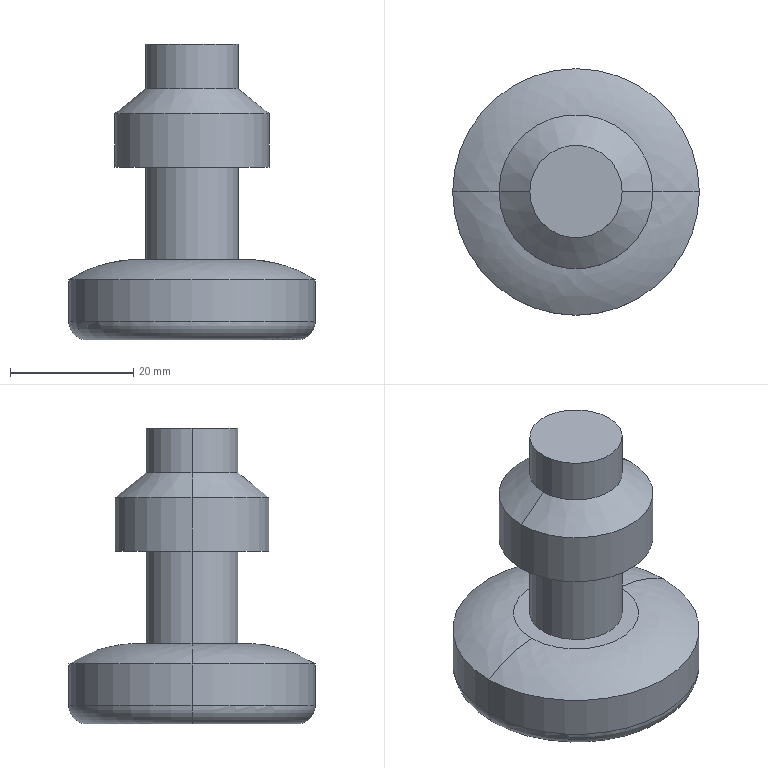Part | STEP file | 1 solid | 18 faces | box 40 x 40 x 48 mm | volume 24355 mm3 | cylinder 8 | plane 4 | torus 2 | other 2 | cone 2 | commonest cylinder face diameters 15 x4 25 x2 40 x2
STEP:
#1=CARTESIAN_POINT('',(0.,0.,0.));
#2=DIRECTION('',(0.,0.,1.));
#3=DIRECTION('',(1.,0.,0.));
#4=AXIS2_PLACEMENT_3D('',#1,#2,#3);
#5=CARTESIAN_POINT('',(-20.,0.,3.));
#6=VERTEX_POINT('',#5);
#7=CARTESIAN_POINT('',(20.,0.,3.));
#8=VERTEX_POINT('',#7);
#9=CARTESIAN_POINT('',(0.,0.,3.));
#10=DIRECTION('',(0.,0.,-1.));
#11=DIRECTION('',(-1.,0.,0.));
#12=AXIS2_PLACEMENT_3D('',#9,#10,#11);
#13=CIRCLE('',#12,20.);
#14=CARTESIAN_POINT('',(0.,0.,3.));
#15=DIRECTION('',(0.,0.,-1.));
#16=DIRECTION('',(-1.,0.,0.));
#17=AXIS2_PLACEMENT_3D('',#14,#15,#16);
#18=TOROIDAL_SURFACE('',#17,17.,3.);
#19=CARTESIAN_POINT('',(0.,0.));
#20=DIRECTION('',(1.,0.));
#21=VECTOR('',#20,1.);
#22=LINE('',#19,#21);
#23=(GEOMETRIC_REPRESENTATION_CONTEXT(2)PARAMETRIC_REPRESENTATION_CONTEXT()REPRESENTATION_CONTEXT('',''));
#24=DEFINITIONAL_REPRESENTATION('',(#22),#23);
#25=PCURVE('',#18,#24);
#26=CARTESIAN_POINT('',(0.,0.,0.));
#27=DIRECTION('',(0.,0.,-1.));
#28=DIRECTION('',(-1.,0.,0.));
#29=AXIS2_PLACEMENT_3D('',#26,#27,#28);
#30=CYLINDRICAL_SURFACE('',#29,20.);
#31=CARTESIAN_POINT('',(0.,-3.));
#32=DIRECTION('',(1.,0.));
#33=VECTOR('',#32,1.);
#34=LINE('',#31,#33);
#35=(GEOMETRIC_REPRESENTATION_CONTEXT(2)PARAMETRIC_REPRESENTATION_CONTEXT()REPRESENTATION_CONTEXT('',''));
#36=DEFINITIONAL_REPRESENTATION('',(#34),#35);
#37=PCURVE('',#30,#36);
#38=SURFACE_CURVE('',#13,(#25,#37),.PCURVE_S1.);
#39=EDGE_CURVE('',#6,#8,#38,.T.);
#40=ORIENTED_EDGE('',*,*,#39,.T.);
#41=CARTESIAN_POINT('',(17.,0.,0.));
#42=VERTEX_POINT('',#41);
#43=CARTESIAN_POINT('',(17.,0.,3.));
#44=DIRECTION('',(0.,1.,0.));
#45=DIRECTION('',(-1.,0.,0.));
#46=AXIS2_PLACEMENT_3D('',#43,#44,#45);
#47=CIRCLE('',#46,3.);
#48=CARTESIAN_POINT('',(3.142,-3.142));
#49=DIRECTION('',(0.,1.));
#50=VECTOR('',#49,1.);
#51=LINE('',#48,#50);
#52=(GEOMETRIC_REPRESENTATION_CONTEXT(2)PARAMETRIC_REPRESENTATION_CONTEXT()REPRESENTATION_CONTEXT('',''));
#53=DEFINITIONAL_REPRESENTATION('',(#51),#52);
#54=PCURVE('',#18,#53);
#55=CARTESIAN_POINT('',(0.,0.,3.));
#56=DIRECTION('',(0.,0.,-1.));
#57=DIRECTION('',(-1.,0.,0.));
#58=AXIS2_PLACEMENT_3D('',#55,#56,#57);
#59=TOROIDAL_SURFACE('',#58,17.,3.);
#60=CARTESIAN_POINT('',(3.142,-3.142));
#61=DIRECTION('',(0.,1.));
#62=VECTOR('',#61,1.);
#63=LINE('',#60,#62);
#64=(GEOMETRIC_REPRESENTATION_CONTEXT(2)PARAMETRIC_REPRESENTATION_CONTEXT()REPRESENTATION_CONTEXT('',''));
#65=DEFINITIONAL_REPRESENTATION('',(#63),#64);
#66=PCURVE('',#59,#65);
#67=SURFACE_CURVE('',#47,(#54,#66),.PCURVE_S1.);
#68=EDGE_CURVE('',#8,#42,#67,.T.);
#69=ORIENTED_EDGE('',*,*,#68,.T.);
#70=CARTESIAN_POINT('',(-17.,0.,0.));
#71=VERTEX_POINT('',#70);
#72=CARTESIAN_POINT('',(0.,0.,0.));
#73=DIRECTION('',(0.,0.,-1.));
#74=DIRECTION('',(-1.,0.,0.));
#75=AXIS2_PLACEMENT_3D('',#72,#73,#74);
#76=CIRCLE('',#75,17.);
#77=CARTESIAN_POINT('',(0.,1.571));
#78=DIRECTION('',(1.,0.));
#79=VECTOR('',#78,1.);
#80=LINE('',#77,#79);
#81=(GEOMETRIC_REPRESENTATION_CONTEXT(2)PARAMETRIC_REPRESENTATION_CONTEXT()REPRESENTATION_CONTEXT('',''));
#82=DEFINITIONAL_REPRESENTATION('',(#80),#81);
#83=PCURVE('',#18,#82);
#84=CARTESIAN_POINT('',(0.,0.,0.));
#85=DIRECTION('',(0.,0.,1.));
#86=DIRECTION('',(1.,0.,0.));
#87=AXIS2_PLACEMENT_3D('',#84,#85,#86);
#88=PLANE('',#87);
#89=CARTESIAN_POINT('',(-17.,0.));
#90=CARTESIAN_POINT('',(-17.,29.445));
#91=CARTESIAN_POINT('',(8.5,14.722));
#92=CARTESIAN_POINT('',(34.,0.));
#93=CARTESIAN_POINT('',(8.5,-14.722));
#94=CARTESIAN_POINT('',(-17.,-29.445));
#95=CARTESIAN_POINT('',(-17.,0.));
#96=(BOUNDED_CURVE()B_SPLINE_CURVE(2,(#89,#90,#91,#92,#93,#94,#95),.UNSPECIFIED.,.T.,.F.)B_SPLINE_CURVE_WITH_KNOTS((1,2,2,2,2,1),(-2.094,0.,2.094,4.189,6.283,8.378),.UNSPECIFIED.)CURVE()GEOMETRIC_REPRESENTATION_ITEM()RATIONAL_B_SPLINE_CURVE((1.,0.5,1.,0.5,1.,0.5,1.))REPRESENTATION_ITEM(''));
#97=(GEOMETRIC_REPRESENTATION_CONTEXT(2)PARAMETRIC_REPRESENTATION_CONTEXT()REPRESENTATION_CONTEXT('',''));
#98=DEFINITIONAL_REPRESENTATION('',(#96),#97);
#99=PCURVE('',#88,#98);
#100=SURFACE_CURVE('',#76,(#83,#99),.PCURVE_S1.);
#101=EDGE_CURVE('',#71,#42,#100,.T.);
#102=ORIENTED_EDGE('',*,*,#101,.F.);
#103=CARTESIAN_POINT('',(-17.,0.,3.));
#104=DIRECTION('',(0.,-1.,0.));
#105=DIRECTION('',(0.,0.,-1.));
#106=AXIS2_PLACEMENT_3D('',#103,#104,#105);
#107=CIRCLE('',#106,3.);
#108=CARTESIAN_POINT('',(0.,-4.712));
#109=DIRECTION('',(0.,1.));
#110=VECTOR('',#109,1.);
#111=LINE('',#108,#110);
#112=(GEOMETRIC_REPRESENTATION_CONTEXT(2)PARAMETRIC_REPRESENTATION_CONTEXT()REPRESENTATION_CONTEXT('',''));
#113=DEFINITIONAL_REPRESENTATION('',(#111),#112);
#114=PCURVE('',#18,#113);
#115=CARTESIAN_POINT('',(6.283,-4.712));
#116=DIRECTION('',(0.,1.));
#117=VECTOR('',#116,1.);
#118=LINE('',#115,#117);
#119=(GEOMETRIC_REPRESENTATION_CONTEXT(2)PARAMETRIC_REPRESENTATION_CONTEXT()REPRESENTATION_CONTEXT('',''));
#120=DEFINITIONAL_REPRESENTATION('',(#118),#119);
#121=PCURVE('',#59,#120);
#122=SURFACE_CURVE('',#107,(#114,#121),.PCURVE_S1.);
#123=EDGE_CURVE('',#6,#71,#122,.T.);
#124=ORIENTED_EDGE('',*,*,#123,.F.);
#125=EDGE_LOOP('',(#40,#69,#102,#124));
#126=FACE_BOUND('',#125,.T.);
#127=ADVANCED_FACE('',(#126),#18,.T.);
#128=CARTESIAN_POINT('',(-20.,0.,9.724));
#129=VERTEX_POINT('',#128);
#130=CARTESIAN_POINT('',(20.,0.,9.724));
#131=VERTEX_POINT('',#130);
#132=CARTESIAN_POINT('',(0.,0.,9.724));
#133=DIRECTION('',(0.,0.,-1.));
#134=DIRECTION('',(-1.,0.,0.));
#135=AXIS2_PLACEMENT_3D('',#132,#133,#134);
#136=CIRCLE('',#135,20.);
#137=CARTESIAN_POINT('',(0.,-9.724));
#138=DIRECTION('',(1.,0.));
#139=VECTOR('',#138,1.);
#140=LINE('',#137,#139);
#141=(GEOMETRIC_REPRESENTATION_CONTEXT(2)PARAMETRIC_REPRESENTATION_CONTEXT()REPRESENTATION_CONTEXT('',''));
#142=DEFINITIONAL_REPRESENTATION('',(#140),#141);
#143=PCURVE('',#30,#142);
#144=CARTESIAN_POINT('',(-10.174,0.,13.));
#145=CARTESIAN_POINT('',(-12.264,0.,12.863));
#146=CARTESIAN_POINT('',(-14.336,0.,12.458));
#147=CARTESIAN_POINT('',(-16.345,0.,11.788));
#148=CARTESIAN_POINT('',(-18.246,0.,10.868));
#149=CARTESIAN_POINT('',(-20.,0.,9.724));
#150=B_SPLINE_CURVE_WITH_KNOTS('',5,(#144,#145,#146,#147,#148,#149),.UNSPECIFIED.,.F.,.F.,(6,6),(4.778,5.291),.PIECEWISE_BEZIER_KNOTS.);
#151=CARTESIAN_POINT('',(0.,0.,-7.382));
#152=DIRECTION('',(0.,0.,-1.));
#153=AXIS1_PLACEMENT('',#151,#152);
#154=SURFACE_OF_REVOLUTION('',#150,#153);
#155=CARTESIAN_POINT('',(0.,5.291));
#156=DIRECTION('',(1.,0.));
#157=VECTOR('',#156,1.);
#158=LINE('',#155,#157);
#159=(GEOMETRIC_REPRESENTATION_CONTEXT(2)PARAMETRIC_REPRESENTATION_CONTEXT()REPRESENTATION_CONTEXT('',''));
#160=DEFINITIONAL_REPRESENTATION('',(#158),#159);
#161=PCURVE('',#154,#160);
#162=SURFACE_CURVE('',#136,(#143,#161),.PCURVE_S1.);
#163=EDGE_CURVE('',#129,#131,#162,.T.);
#164=ORIENTED_EDGE('',*,*,#163,.T.);
#165=CARTESIAN_POINT('',(20.,0.,0.));
#166=DIRECTION('',(0.,0.,-1.));
#167=VECTOR('',#166,1.);
#168=LINE('',#165,#167);
#169=CARTESIAN_POINT('',(3.142,0.));
#170=DIRECTION('',(0.,1.));
#171=VECTOR('',#170,1.);
#172=LINE('',#169,#171);
#173=(GEOMETRIC_REPRESENTATION_CONTEXT(2)PARAMETRIC_REPRESENTATION_CONTEXT()REPRESENTATION_CONTEXT('',''));
#174=DEFINITIONAL_REPRESENTATION('',(#172),#173);
#175=PCURVE('',#30,#174);
#176=CARTESIAN_POINT('',(0.,0.,0.));
#177=DIRECTION('',(0.,0.,-1.));
#178=DIRECTION('',(-1.,0.,0.));
#179=AXIS2_PLACEMENT_3D('',#176,#177,#178);
#180=CYLINDRICAL_SURFACE('',#179,20.);
#181=CARTESIAN_POINT('',(3.142,0.));
#182=DIRECTION('',(0.,1.));
#183=VECTOR('',#182,1.);
#184=LINE('',#181,#183);
#185=(GEOMETRIC_REPRESENTATION_CONTEXT(2)PARAMETRIC_REPRESENTATION_CONTEXT()REPRESENTATION_CONTEXT('',''));
#186=DEFINITIONAL_REPRESENTATION('',(#184),#185);
#187=PCURVE('',#180,#186);
#188=SURFACE_CURVE('',#168,(#175,#187),.PCURVE_S1.);
#189=EDGE_CURVE('',#131,#8,#188,.T.);
#190=ORIENTED_EDGE('',*,*,#189,.T.);
#191=ORIENTED_EDGE('',*,*,#39,.F.);
#192=CARTESIAN_POINT('',(-20.,0.,0.));
#193=DIRECTION('',(0.,0.,-1.));
#194=VECTOR('',#193,1.);
#195=LINE('',#192,#194);
#196=CARTESIAN_POINT('',(0.,0.));
#197=DIRECTION('',(0.,1.));
#198=VECTOR('',#197,1.);
#199=LINE('',#196,#198);
#200=(GEOMETRIC_REPRESENTATION_CONTEXT(2)PARAMETRIC_REPRESENTATION_CONTEXT()REPRESENTATION_CONTEXT('',''));
#201=DEFINITIONAL_REPRESENTATION('',(#199),#200);
#202=PCURVE('',#30,#201);
#203=CARTESIAN_POINT('',(6.283,0.));
#204=DIRECTION('',(0.,1.));
#205=VECTOR('',#204,1.);
#206=LINE('',#203,#205);
#207=(GEOMETRIC_REPRESENTATION_CONTEXT(2)PARAMETRIC_REPRESENTATION_CONTEXT()REPRESENTATION_CONTEXT('',''));
#208=DEFINITIONAL_REPRESENTATION('',(#206),#207);
#209=PCURVE('',#180,#208);
#210=SURFACE_CURVE('',#195,(#202,#209),.PCURVE_S1.);
#211=EDGE_CURVE('',#129,#6,#210,.T.);
#212=ORIENTED_EDGE('',*,*,#211,.F.);
#213=EDGE_LOOP('',(#164,#190,#191,#212));
#214=FACE_BOUND('',#213,.T.);
#215=ADVANCED_FACE('',(#214),#30,.T.);
#216=CARTESIAN_POINT('',(-10.174,0.,13.));
#217=VERTEX_POINT('',#216);
#218=CARTESIAN_POINT('',(10.174,0.,13.));
#219=VERTEX_POINT('',#218);
#220=CARTESIAN_POINT('',(0.,0.,13.));
#221=DIRECTION('',(0.,0.,-1.));
#222=DIRECTION('',(-1.,0.,0.));
#223=AXIS2_PLACEMENT_3D('',#220,#221,#222);
#224=CIRCLE('',#223,10.174);
#225=CARTESIAN_POINT('',(0.,4.778));
#226=DIRECTION('',(1.,0.));
#227=VECTOR('',#226,1.);
#228=LINE('',#225,#227);
#229=(GEOMETRIC_REPRESENTATION_CONTEXT(2)PARAMETRIC_REPRESENTATION_CONTEXT()REPRESENTATION_CONTEXT('',''));
#230=DEFINITIONAL_REPRESENTATION('',(#228),#229);
#231=PCURVE('',#154,#230);
#232=CARTESIAN_POINT('',(10.174,0.,13.));
#233=DIRECTION('',(0.,0.,-1.));
#234=DIRECTION('',(-1.,0.,0.));
#235=AXIS2_PLACEMENT_3D('',#232,#233,#234);
#236=PLANE('',#235);
#237=CARTESIAN_POINT('',(10.174,0.));
#238=DIRECTION('',(1.,0.));
#239=AXIS2_PLACEMENT_2D('',#237,#238);
#240=CIRCLE('',#239,10.174);
#241=(GEOMETRIC_REPRESENTATION_CONTEXT(2)PARAMETRIC_REPRESENTATION_CONTEXT()REPRESENTATION_CONTEXT('',''));
#242=DEFINITIONAL_REPRESENTATION('',(#240),#241);
#243=PCURVE('',#236,#242);
#244=SURFACE_CURVE('',#224,(#231,#243),.PCURVE_S1.);
#245=EDGE_CURVE('',#217,#219,#244,.T.);
#246=ORIENTED_EDGE('',*,*,#245,.T.);
#247=CARTESIAN_POINT('',(8.837,0.,-7.382));
#248=DIRECTION('',(0.,1.,0.));
#249=DIRECTION('',(-1.,0.,0.));
#250=AXIS2_PLACEMENT_3D('',#247,#248,#249);
#251=CIRCLE('',#250,20.426);
#252=CARTESIAN_POINT('',(3.142,3.142));
#253=DIRECTION('',(0.,1.));
#254=VECTOR('',#253,1.);
#255=LINE('',#252,#254);
#256=(GEOMETRIC_REPRESENTATION_CONTEXT(2)PARAMETRIC_REPRESENTATION_CONTEXT()REPRESENTATION_CONTEXT('',''));
#257=DEFINITIONAL_REPRESENTATION('',(#255),#256);
#258=PCURVE('',#154,#257);
#259=CARTESIAN_POINT('',(-10.174,0.,13.));
#260=CARTESIAN_POINT('',(-12.264,0.,12.863));
#261=CARTESIAN_POINT('',(-14.336,0.,12.458));
#262=CARTESIAN_POINT('',(-16.345,0.,11.788));
#263=CARTESIAN_POINT('',(-18.246,0.,10.868));
#264=CARTESIAN_POINT('',(-20.,0.,9.724));
#265=B_SPLINE_CURVE_WITH_KNOTS('',5,(#259,#260,#261,#262,#263,#264),.UNSPECIFIED.,.F.,.F.,(6,6),(4.778,5.291),.PIECEWISE_BEZIER_KNOTS.);
#266=CARTESIAN_POINT('',(0.,0.,-7.382));
#267=DIRECTION('',(0.,0.,-1.));
#268=AXIS1_PLACEMENT('',#266,#267);
#269=SURFACE_OF_REVOLUTION('',#265,#268);
#270=CARTESIAN_POINT('',(3.142,3.142));
#271=DIRECTION('',(0.,1.));
#272=VECTOR('',#271,1.);
#273=LINE('',#270,#272);
#274=(GEOMETRIC_REPRESENTATION_CONTEXT(2)PARAMETRIC_REPRESENTATION_CONTEXT()REPRESENTATION_CONTEXT('',''));
#275=DEFINITIONAL_REPRESENTATION('',(#273),#274);
#276=PCURVE('',#269,#275);
#277=SURFACE_CURVE('',#251,(#258,#276),.PCURVE_S1.);
#278=EDGE_CURVE('',#219,#131,#277,.T.);
#279=ORIENTED_EDGE('',*,*,#278,.T.);
#280=ORIENTED_EDGE('',*,*,#163,.F.);
#281=CARTESIAN_POINT('',(-8.837,0.,-7.382));
#282=DIRECTION('',(0.,-1.,0.));
#283=DIRECTION('',(0.,0.,-1.));
#284=AXIS2_PLACEMENT_3D('',#281,#282,#283);
#285=CIRCLE('',#284,20.426);
#286=CARTESIAN_POINT('',(0.,1.571));
#287=DIRECTION('',(0.,1.));
#288=VECTOR('',#287,1.);
#289=LINE('',#286,#288);
#290=(GEOMETRIC_REPRESENTATION_CONTEXT(2)PARAMETRIC_REPRESENTATION_CONTEXT()REPRESENTATION_CONTEXT('',''));
#291=DEFINITIONAL_REPRESENTATION('',(#289),#290);
#292=PCURVE('',#154,#291);
#293=CARTESIAN_POINT('',(6.283,1.571));
#294=DIRECTION('',(0.,1.));
#295=VECTOR('',#294,1.);
#296=LINE('',#293,#295);
#297=(GEOMETRIC_REPRESENTATION_CONTEXT(2)PARAMETRIC_REPRESENTATION_CONTEXT()REPRESENTATION_CONTEXT('',''));
#298=DEFINITIONAL_REPRESENTATION('',(#296),#297);
#299=PCURVE('',#269,#298);
#300=SURFACE_CURVE('',#285,(#292,#299),.PCURVE_S1.);
#301=EDGE_CURVE('',#217,#129,#300,.T.);
#302=ORIENTED_EDGE('',*,*,#301,.F.);
#303=EDGE_LOOP('',(#246,#279,#280,#302));
#304=FACE_BOUND('',#303,.T.);
#305=ADVANCED_FACE('',(#304),#154,.T.);
#306=CARTESIAN_POINT('',(-7.5,0.,28.));
#307=VERTEX_POINT('',#306);
#308=CARTESIAN_POINT('',(7.5,0.,28.));
#309=VERTEX_POINT('',#308);
#310=CARTESIAN_POINT('',(0.,0.,28.));
#311=DIRECTION('',(0.,0.,-1.));
#312=DIRECTION('',(-1.,0.,0.));
#313=AXIS2_PLACEMENT_3D('',#310,#311,#312);
#314=CIRCLE('',#313,7.5);
#315=CARTESIAN_POINT('',(0.,0.,0.));
#316=DIRECTION('',(0.,0.,-1.));
#317=DIRECTION('',(-1.,0.,0.));
#318=AXIS2_PLACEMENT_3D('',#315,#316,#317);
#319=CYLINDRICAL_SURFACE('',#318,7.5);
#320=CARTESIAN_POINT('',(0.,-28.));
#321=DIRECTION('',(1.,0.));
#322=VECTOR('',#321,1.);
#323=LINE('',#320,#322);
#324=(GEOMETRIC_REPRESENTATION_CONTEXT(2)PARAMETRIC_REPRESENTATION_CONTEXT()REPRESENTATION_CONTEXT('',''));
#325=DEFINITIONAL_REPRESENTATION('',(#323),#324);
#326=PCURVE('',#319,#325);
#327=CARTESIAN_POINT('',(7.5,0.,28.));
#328=DIRECTION('',(0.,0.,1.));
#329=DIRECTION('',(1.,0.,0.));
#330=AXIS2_PLACEMENT_3D('',#327,#328,#329);
#331=PLANE('',#330);
#332=CARTESIAN_POINT('',(-15.,0.));
#333=CARTESIAN_POINT('',(-15.,12.99));
#334=CARTESIAN_POINT('',(-3.75,6.495));
#335=CARTESIAN_POINT('',(7.5,0.));
#336=CARTESIAN_POINT('',(-3.75,-6.495));
#337=CARTESIAN_POINT('',(-15.,-12.99));
#338=CARTESIAN_POINT('',(-15.,0.));
#339=(BOUNDED_CURVE()B_SPLINE_CURVE(2,(#332,#333,#334,#335,#336,#337,#338),.UNSPECIFIED.,.T.,.F.)B_SPLINE_CURVE_WITH_KNOTS((1,2,2,2,2,1),(-2.094,0.,2.094,4.189,6.283,8.378),.UNSPECIFIED.)CURVE()GEOMETRIC_REPRESENTATION_ITEM()RATIONAL_B_SPLINE_CURVE((1.,0.5,1.,0.5,1.,0.5,1.))REPRESENTATION_ITEM(''));
#340=(GEOMETRIC_REPRESENTATION_CONTEXT(2)PARAMETRIC_REPRESENTATION_CONTEXT()REPRESENTATION_CONTEXT('',''));
#341=DEFINITIONAL_REPRESENTATION('',(#339),#340);
#342=PCURVE('',#331,#341);
#343=SURFACE_CURVE('',#314,(#326,#342),.PCURVE_S1.);
#344=EDGE_CURVE('',#307,#309,#343,.T.);
#345=ORIENTED_EDGE('',*,*,#344,.T.);
#346=CARTESIAN_POINT('',(7.5,0.,13.));
#347=VERTEX_POINT('',#346);
#348=CARTESIAN_POINT('',(7.5,0.,0.));
#349=DIRECTION('',(0.,0.,-1.));
#350=VECTOR('',#349,1.);
#351=LINE('',#348,#350);
#352=CARTESIAN_POINT('',(3.142,0.));
#353=DIRECTION('',(0.,1.));
#354=VECTOR('',#353,1.);
#355=LINE('',#352,#354);
#356=(GEOMETRIC_REPRESENTATION_CONTEXT(2)PARAMETRIC_REPRESENTATION_CONTEXT()REPRESENTATION_CONTEXT('',''));
#357=DEFINITIONAL_REPRESENTATION('',(#355),#356);
#358=PCURVE('',#319,#357);
#359=CARTESIAN_POINT('',(0.,0.,0.));
#360=DIRECTION('',(0.,0.,-1.));
#361=DIRECTION('',(-1.,0.,0.));
#362=AXIS2_PLACEMENT_3D('',#359,#360,#361);
#363=CYLINDRICAL_SURFACE('',#362,7.5);
#364=CARTESIAN_POINT('',(3.142,0.));
#365=DIRECTION('',(0.,1.));
#366=VECTOR('',#365,1.);
#367=LINE('',#364,#366);
#368=(GEOMETRIC_REPRESENTATION_CONTEXT(2)PARAMETRIC_REPRESENTATION_CONTEXT()REPRESENTATION_CONTEXT('',''));
#369=DEFINITIONAL_REPRESENTATION('',(#367),#368);
#370=PCURVE('',#363,#369);
#371=SURFACE_CURVE('',#351,(#358,#370),.PCURVE_S1.);
#372=EDGE_CURVE('',#309,#347,#371,.T.);
#373=ORIENTED_EDGE('',*,*,#372,.T.);
#374=CARTESIAN_POINT('',(-7.5,0.,13.));
#375=VERTEX_POINT('',#374);
#376=CARTESIAN_POINT('',(0.,0.,13.));
#377=DIRECTION('',(0.,0.,-1.));
#378=DIRECTION('',(-1.,0.,0.));
#379=AXIS2_PLACEMENT_3D('',#376,#377,#378);
#380=CIRCLE('',#379,7.5);
#381=CARTESIAN_POINT('',(0.,-13.));
#382=DIRECTION('',(1.,0.));
#383=VECTOR('',#382,1.);
#384=LINE('',#381,#383);
#385=(GEOMETRIC_REPRESENTATION_CONTEXT(2)PARAMETRIC_REPRESENTATION_CONTEXT()REPRESENTATION_CONTEXT('',''));
#386=DEFINITIONAL_REPRESENTATION('',(#384),#385);
#387=PCURVE('',#319,#386);
#388=CARTESIAN_POINT('',(10.174,0.));
#389=DIRECTION('',(1.,0.));
#390=AXIS2_PLACEMENT_2D('',#388,#389);
#391=CIRCLE('',#390,7.5);
#392=(GEOMETRIC_REPRESENTATION_CONTEXT(2)PARAMETRIC_REPRESENTATION_CONTEXT()REPRESENTATION_CONTEXT('',''));
#393=DEFINITIONAL_REPRESENTATION('',(#391),#392);
#394=PCURVE('',#236,#393);
#395=SURFACE_CURVE('',#380,(#387,#394),.PCURVE_S1.);
#396=EDGE_CURVE('',#375,#347,#395,.T.);
#397=ORIENTED_EDGE('',*,*,#396,.F.);
#398=CARTESIAN_POINT('',(-7.5,0.,0.));
#399=DIRECTION('',(0.,0.,-1.));
#400=VECTOR('',#399,1.);
#401=LINE('',#398,#400);
#402=CARTESIAN_POINT('',(0.,0.));
#403=DIRECTION('',(0.,1.));
#404=VECTOR('',#403,1.);
#405=LINE('',#402,#404);
#406=(GEOMETRIC_REPRESENTATION_CONTEXT(2)PARAMETRIC_REPRESENTATION_CONTEXT()REPRESENTATION_CONTEXT('',''));
#407=DEFINITIONAL_REPRESENTATION('',(#405),#406);
#408=PCURVE('',#319,#407);
#409=CARTESIAN_POINT('',(6.283,0.));
#410=DIRECTION('',(0.,1.));
#411=VECTOR('',#410,1.);
#412=LINE('',#409,#411);
#413=(GEOMETRIC_REPRESENTATION_CONTEXT(2)PARAMETRIC_REPRESENTATION_CONTEXT()REPRESENTATION_CONTEXT('',''));
#414=DEFINITIONAL_REPRESENTATION('',(#412),#413);
#415=PCURVE('',#363,#414);
#416=SURFACE_CURVE('',#401,(#408,#415),.PCURVE_S1.);
#417=EDGE_CURVE('',#307,#375,#416,.T.);
#418=ORIENTED_EDGE('',*,*,#417,.F.);
#419=EDGE_LOOP('',(#345,#373,#397,#418));
#420=FACE_BOUND('',#419,.T.);
#421=ADVANCED_FACE('',(#420),#319,.T.);
#422=CARTESIAN_POINT('',(-12.5,0.,36.732));
#423=VERTEX_POINT('',#422);
#424=CARTESIAN_POINT('',(12.5,0.,36.732));
#425=VERTEX_POINT('',#424);
#426=CARTESIAN_POINT('',(0.,0.,36.732));
#427=DIRECTION('',(0.,0.,-1.));
#428=DIRECTION('',(-1.,0.,0.));
#429=AXIS2_PLACEMENT_3D('',#426,#427,#428);
#430=CIRCLE('',#429,12.5);
#431=CARTESIAN_POINT('',(0.,0.,0.));
#432=DIRECTION('',(0.,0.,-1.));
#433=DIRECTION('',(-1.,0.,0.));
#434=AXIS2_PLACEMENT_3D('',#431,#432,#433);
#435=CYLINDRICAL_SURFACE('',#434,12.5);
#436=CARTESIAN_POINT('',(0.,-36.732));
#437=DIRECTION('',(1.,0.));
#438=VECTOR('',#437,1.);
#439=LINE('',#436,#438);
#440=(GEOMETRIC_REPRESENTATION_CONTEXT(2)PARAMETRIC_REPRESENTATION_CONTEXT()REPRESENTATION_CONTEXT('',''));
#441=DEFINITIONAL_REPRESENTATION('',(#439),#440);
#442=PCURVE('',#435,#441);
#443=CARTESIAN_POINT('',(0.,0.,40.733));
#444=DIRECTION('',(0.,0.,-1.));
#445=DIRECTION('',(-1.,0.,0.));
#446=AXIS2_PLACEMENT_3D('',#443,#444,#445);
#447=CONICAL_SURFACE('',#446,7.5,0.8959);
#448=CARTESIAN_POINT('',(0.,4.001));
#449=DIRECTION('',(1.,0.));
#450=VECTOR('',#449,1.);
#451=LINE('',#448,#450);
#452=(GEOMETRIC_REPRESENTATION_CONTEXT(2)PARAMETRIC_REPRESENTATION_CONTEXT()REPRESENTATION_CONTEXT('',''));
#453=DEFINITIONAL_REPRESENTATION('',(#451),#452);
#454=PCURVE('',#447,#453);
#455=SURFACE_CURVE('',#430,(#442,#454),.PCURVE_S1.);
#456=EDGE_CURVE('',#423,#425,#455,.T.);
#457=ORIENTED_EDGE('',*,*,#456,.T.);
#458=CARTESIAN_POINT('',(12.5,0.,28.));
#459=VERTEX_POINT('',#458);
#460=CARTESIAN_POINT('',(12.5,0.,0.));
#461=DIRECTION('',(0.,0.,-1.));
#462=VECTOR('',#461,1.);
#463=LINE('',#460,#462);
#464=CARTESIAN_POINT('',(3.142,0.));
#465=DIRECTION('',(0.,1.));
#466=VECTOR('',#465,1.);
#467=LINE('',#464,#466);
#468=(GEOMETRIC_REPRESENTATION_CONTEXT(2)PARAMETRIC_REPRESENTATION_CONTEXT()REPRESENTATION_CONTEXT('',''));
#469=DEFINITIONAL_REPRESENTATION('',(#467),#468);
#470=PCURVE('',#435,#469);
#471=CARTESIAN_POINT('',(0.,0.,0.));
#472=DIRECTION('',(0.,0.,-1.));
#473=DIRECTION('',(-1.,0.,0.));
#474=AXIS2_PLACEMENT_3D('',#471,#472,#473);
#475=CYLINDRICAL_SURFACE('',#474,12.5);
#476=CARTESIAN_POINT('',(3.142,0.));
#477=DIRECTION('',(0.,1.));
#478=VECTOR('',#477,1.);
#479=LINE('',#476,#478);
#480=(GEOMETRIC_REPRESENTATION_CONTEXT(2)PARAMETRIC_REPRESENTATION_CONTEXT()REPRESENTATION_CONTEXT('',''));
#481=DEFINITIONAL_REPRESENTATION('',(#479),#480);
#482=PCURVE('',#475,#481);
#483=SURFACE_CURVE('',#463,(#470,#482),.PCURVE_S1.);
#484=EDGE_CURVE('',#425,#459,#483,.T.);
#485=ORIENTED_EDGE('',*,*,#484,.T.);
#486=CARTESIAN_POINT('',(-12.5,0.,28.));
#487=VERTEX_POINT('',#486);
#488=CARTESIAN_POINT('',(0.,0.,28.));
#489=DIRECTION('',(0.,0.,-1.));
#490=DIRECTION('',(-1.,0.,0.));
#491=AXIS2_PLACEMENT_3D('',#488,#489,#490);
#492=CIRCLE('',#491,12.5);
#493=CARTESIAN_POINT('',(0.,-28.));
#494=DIRECTION('',(1.,0.));
#495=VECTOR('',#494,1.);
#496=LINE('',#493,#495);
#497=(GEOMETRIC_REPRESENTATION_CONTEXT(2)PARAMETRIC_REPRESENTATION_CONTEXT()REPRESENTATION_CONTEXT('',''));
#498=DEFINITIONAL_REPRESENTATION('',(#496),#497);
#499=PCURVE('',#435,#498);
#500=CARTESIAN_POINT('',(-20.,0.));
#501=CARTESIAN_POINT('',(-20.,21.651));
#502=CARTESIAN_POINT('',(-1.25,10.825));
#503=CARTESIAN_POINT('',(17.5,0.));
#504=CARTESIAN_POINT('',(-1.25,-10.825));
#505=CARTESIAN_POINT('',(-20.,-21.651));
#506=CARTESIAN_POINT('',(-20.,0.));
#507=(BOUNDED_CURVE()B_SPLINE_CURVE(2,(#500,#501,#502,#503,#504,#505,#506),.UNSPECIFIED.,.T.,.F.)B_SPLINE_CURVE_WITH_KNOTS((1,2,2,2,2,1),(-2.094,0.,2.094,4.189,6.283,8.378),.UNSPECIFIED.)CURVE()GEOMETRIC_REPRESENTATION_ITEM()RATIONAL_B_SPLINE_CURVE((1.,0.5,1.,0.5,1.,0.5,1.))REPRESENTATION_ITEM(''));
#508=(GEOMETRIC_REPRESENTATION_CONTEXT(2)PARAMETRIC_REPRESENTATION_CONTEXT()REPRESENTATION_CONTEXT('',''));
#509=DEFINITIONAL_REPRESENTATION('',(#507),#508);
#510=PCURVE('',#331,#509);
#511=SURFACE_CURVE('',#492,(#499,#510),.PCURVE_S1.);
#512=EDGE_CURVE('',#487,#459,#511,.T.);
#513=ORIENTED_EDGE('',*,*,#512,.F.);
#514=CARTESIAN_POINT('',(-12.5,0.,0.));
#515=DIRECTION('',(0.,0.,-1.));
#516=VECTOR('',#515,1.);
#517=LINE('',#514,#516);
#518=CARTESIAN_POINT('',(0.,0.));
#519=DIRECTION('',(0.,1.));
#520=VECTOR('',#519,1.);
#521=LINE('',#518,#520);
#522=(GEOMETRIC_REPRESENTATION_CONTEXT(2)PARAMETRIC_REPRESENTATION_CONTEXT()REPRESENTATION_CONTEXT('',''));
#523=DEFINITIONAL_REPRESENTATION('',(#521),#522);
#524=PCURVE('',#435,#523);
#525=CARTESIAN_POINT('',(6.283,0.));
#526=DIRECTION('',(0.,1.));
#527=VECTOR('',#526,1.);
#528=LINE('',#525,#527);
#529=(GEOMETRIC_REPRESENTATION_CONTEXT(2)PARAMETRIC_REPRESENTATION_CONTEXT()REPRESENTATION_CONTEXT('',''));
#530=DEFINITIONAL_REPRESENTATION('',(#528),#529);
#531=PCURVE('',#475,#530);
#532=SURFACE_CURVE('',#517,(#524,#531),.PCURVE_S1.);
#533=EDGE_CURVE('',#423,#487,#532,.T.);
#534=ORIENTED_EDGE('',*,*,#533,.F.);
#535=EDGE_LOOP('',(#457,#485,#513,#534));
#536=FACE_BOUND('',#535,.T.);
#537=ADVANCED_FACE('',(#536),#435,.T.);
#538=CARTESIAN_POINT('',(-7.5,0.,40.733));
#539=VERTEX_POINT('',#538);
#540=CARTESIAN_POINT('',(7.5,0.,40.733));
#541=VERTEX_POINT('',#540);
#542=CARTESIAN_POINT('',(0.,0.,40.733));
#543=DIRECTION('',(0.,0.,-1.));
#544=DIRECTION('',(-1.,0.,0.));
#545=AXIS2_PLACEMENT_3D('',#542,#543,#544);
#546=CIRCLE('',#545,7.5);
#547=CARTESIAN_POINT('',(0.,0.));
#548=DIRECTION('',(1.,0.));
#549=VECTOR('',#548,1.);
#550=LINE('',#547,#549);
#551=(GEOMETRIC_REPRESENTATION_CONTEXT(2)PARAMETRIC_REPRESENTATION_CONTEXT()REPRESENTATION_CONTEXT('',''));
#552=DEFINITIONAL_REPRESENTATION('',(#550),#551);
#553=PCURVE('',#447,#552);
#554=CARTESIAN_POINT('',(0.,0.,0.));
#555=DIRECTION('',(0.,0.,-1.));
#556=DIRECTION('',(-1.,0.,0.));
#557=AXIS2_PLACEMENT_3D('',#554,#555,#556);
#558=CYLINDRICAL_SURFACE('',#557,7.5);
#559=CARTESIAN_POINT('',(0.,-40.733));
#560=DIRECTION('',(1.,0.));
#561=VECTOR('',#560,1.);
#562=LINE('',#559,#561);
#563=(GEOMETRIC_REPRESENTATION_CONTEXT(2)PARAMETRIC_REPRESENTATION_CONTEXT()REPRESENTATION_CONTEXT('',''));
#564=DEFINITIONAL_REPRESENTATION('',(#562),#563);
#565=PCURVE('',#558,#564);
#566=SURFACE_CURVE('',#546,(#553,#565),.PCURVE_S1.);
#567=EDGE_CURVE('',#539,#541,#566,.T.);
#568=ORIENTED_EDGE('',*,*,#567,.T.);
#569=CARTESIAN_POINT('',(7.5,0.,40.733));
#570=DIRECTION('',(0.7808,0.,-0.6248));
#571=VECTOR('',#570,1.);
#572=LINE('',#569,#571);
#573=CARTESIAN_POINT('',(3.142,0.));
#574=DIRECTION('',(0.,1.));
#575=VECTOR('',#574,1.);
#576=LINE('',#573,#575);
#577=(GEOMETRIC_REPRESENTATION_CONTEXT(2)PARAMETRIC_REPRESENTATION_CONTEXT()REPRESENTATION_CONTEXT('',''));
#578=DEFINITIONAL_REPRESENTATION('',(#576),#577);
#579=PCURVE('',#447,#578);
#580=CARTESIAN_POINT('',(0.,0.,40.733));
#581=DIRECTION('',(0.,0.,-1.));
#582=DIRECTION('',(-1.,0.,0.));
#583=AXIS2_PLACEMENT_3D('',#580,#581,#582);
#584=CONICAL_SURFACE('',#583,7.5,0.8959);
#585=CARTESIAN_POINT('',(3.142,0.));
#586=DIRECTION('',(0.,1.));
#587=VECTOR('',#586,1.);
#588=LINE('',#585,#587);
#589=(GEOMETRIC_REPRESENTATION_CONTEXT(2)PARAMETRIC_REPRESENTATION_CONTEXT()REPRESENTATION_CONTEXT('',''));
#590=DEFINITIONAL_REPRESENTATION('',(#588),#589);
#591=PCURVE('',#584,#590);
#592=SURFACE_CURVE('',#572,(#579,#591),.PCURVE_S1.);
#593=EDGE_CURVE('',#541,#425,#592,.T.);
#594=ORIENTED_EDGE('',*,*,#593,.T.);
#595=ORIENTED_EDGE('',*,*,#456,.F.);
#596=CARTESIAN_POINT('',(-7.5,0.,40.733));
#597=DIRECTION('',(-0.7808,0.,-0.6248));
#598=VECTOR('',#597,1.);
#599=LINE('',#596,#598);
#600=CARTESIAN_POINT('',(0.,0.));
#601=DIRECTION('',(0.,1.));
#602=VECTOR('',#601,1.);
#603=LINE('',#600,#602);
#604=(GEOMETRIC_REPRESENTATION_CONTEXT(2)PARAMETRIC_REPRESENTATION_CONTEXT()REPRESENTATION_CONTEXT('',''));
#605=DEFINITIONAL_REPRESENTATION('',(#603),#604);
#606=PCURVE('',#447,#605);
#607=CARTESIAN_POINT('',(6.283,0.));
#608=DIRECTION('',(0.,1.));
#609=VECTOR('',#608,1.);
#610=LINE('',#607,#609);
#611=(GEOMETRIC_REPRESENTATION_CONTEXT(2)PARAMETRIC_REPRESENTATION_CONTEXT()REPRESENTATION_CONTEXT('',''));
#612=DEFINITIONAL_REPRESENTATION('',(#610),#611);
#613=PCURVE('',#584,#612);
#614=SURFACE_CURVE('',#599,(#606,#613),.PCURVE_S1.);
#615=EDGE_CURVE('',#539,#423,#614,.T.);
#616=ORIENTED_EDGE('',*,*,#615,.F.);
#617=EDGE_LOOP('',(#568,#594,#595,#616));
#618=FACE_BOUND('',#617,.T.);
#619=ADVANCED_FACE('',(#618),#447,.T.);
#620=CARTESIAN_POINT('',(-7.5,0.,48.));
#621=VERTEX_POINT('',#620);
#622=CARTESIAN_POINT('',(7.5,0.,48.));
#623=VERTEX_POINT('',#622);
#624=CARTESIAN_POINT('',(0.,0.,48.));
#625=DIRECTION('',(0.,0.,-1.));
#626=DIRECTION('',(-1.,0.,0.));
#627=AXIS2_PLACEMENT_3D('',#624,#625,#626);
#628=CIRCLE('',#627,7.5);
#629=CARTESIAN_POINT('',(0.,-48.));
#630=DIRECTION('',(1.,0.));
#631=VECTOR('',#630,1.);
#632=LINE('',#629,#631);
#633=(GEOMETRIC_REPRESENTATION_CONTEXT(2)PARAMETRIC_REPRESENTATION_CONTEXT()REPRESENTATION_CONTEXT('',''));
#634=DEFINITIONAL_REPRESENTATION('',(#632),#633);
#635=PCURVE('',#558,#634);
#636=CARTESIAN_POINT('',(7.5,0.,48.));
#637=DIRECTION('',(0.,0.,-1.));
#638=DIRECTION('',(-1.,0.,0.));
#639=AXIS2_PLACEMENT_3D('',#636,#637,#638);
#640=PLANE('',#639);
#641=CARTESIAN_POINT('',(7.5,0.));
#642=DIRECTION('',(1.,0.));
#643=AXIS2_PLACEMENT_2D('',#641,#642);
#644=CIRCLE('',#643,7.5);
#645=(GEOMETRIC_REPRESENTATION_CONTEXT(2)PARAMETRIC_REPRESENTATION_CONTEXT()REPRESENTATION_CONTEXT('',''));
#646=DEFINITIONAL_REPRESENTATION('',(#644),#645);
#647=PCURVE('',#640,#646);
#648=SURFACE_CURVE('',#628,(#635,#647),.PCURVE_S1.);
#649=EDGE_CURVE('',#621,#623,#648,.T.);
#650=ORIENTED_EDGE('',*,*,#649,.T.);
#651=CARTESIAN_POINT('',(7.5,0.,0.));
#652=DIRECTION('',(0.,0.,-1.));
#653=VECTOR('',#652,1.);
#654=LINE('',#651,#653);
#655=CARTESIAN_POINT('',(3.142,0.));
#656=DIRECTION('',(0.,1.));
#657=VECTOR('',#656,1.);
#658=LINE('',#655,#657);
#659=(GEOMETRIC_REPRESENTATION_CONTEXT(2)PARAMETRIC_REPRESENTATION_CONTEXT()REPRESENTATION_CONTEXT('',''));
#660=DEFINITIONAL_REPRESENTATION('',(#658),#659);
#661=PCURVE('',#558,#660);
#662=CARTESIAN_POINT('',(0.,0.,0.));
#663=DIRECTION('',(0.,0.,-1.));
#664=DIRECTION('',(-1.,0.,0.));
#665=AXIS2_PLACEMENT_3D('',#662,#663,#664);
#666=CYLINDRICAL_SURFACE('',#665,7.5);
#667=CARTESIAN_POINT('',(3.142,0.));
#668=DIRECTION('',(0.,1.));
#669=VECTOR('',#668,1.);
#670=LINE('',#667,#669);
#671=(GEOMETRIC_REPRESENTATION_CONTEXT(2)PARAMETRIC_REPRESENTATION_CONTEXT()REPRESENTATION_CONTEXT('',''));
#672=DEFINITIONAL_REPRESENTATION('',(#670),#671);
#673=PCURVE('',#666,#672);
#674=SURFACE_CURVE('',#654,(#661,#673),.PCURVE_S1.);
#675=EDGE_CURVE('',#623,#541,#674,.T.);
#676=ORIENTED_EDGE('',*,*,#675,.T.);
#677=ORIENTED_EDGE('',*,*,#567,.F.);
#678=CARTESIAN_POINT('',(-7.5,0.,0.));
#679=DIRECTION('',(0.,0.,-1.));
#680=VECTOR('',#679,1.);
#681=LINE('',#678,#680);
#682=CARTESIAN_POINT('',(0.,0.));
#683=DIRECTION('',(0.,1.));
#684=VECTOR('',#683,1.);
#685=LINE('',#682,#684);
#686=(GEOMETRIC_REPRESENTATION_CONTEXT(2)PARAMETRIC_REPRESENTATION_CONTEXT()REPRESENTATION_CONTEXT('',''));
#687=DEFINITIONAL_REPRESENTATION('',(#685),#686);
#688=PCURVE('',#558,#687);
#689=CARTESIAN_POINT('',(6.283,0.));
#690=DIRECTION('',(0.,1.));
#691=VECTOR('',#690,1.);
#692=LINE('',#689,#691);
#693=(GEOMETRIC_REPRESENTATION_CONTEXT(2)PARAMETRIC_REPRESENTATION_CONTEXT()REPRESENTATION_CONTEXT('',''));
#694=DEFINITIONAL_REPRESENTATION('',(#692),#693);
#695=PCURVE('',#666,#694);
#696=SURFACE_CURVE('',#681,(#688,#695),.PCURVE_S1.);
#697=EDGE_CURVE('',#621,#539,#696,.T.);
#698=ORIENTED_EDGE('',*,*,#697,.F.);
#699=EDGE_LOOP('',(#650,#676,#677,#698));
#700=FACE_BOUND('',#699,.T.);
#701=ADVANCED_FACE('',(#700),#558,.T.);
#702=ORIENTED_EDGE('',*,*,#649,.F.);
#703=CARTESIAN_POINT('',(0.,0.,48.));
#704=DIRECTION('',(0.,0.,-1.));
#705=DIRECTION('',(-1.,0.,0.));
#706=AXIS2_PLACEMENT_3D('',#703,#704,#705);
#707=CIRCLE('',#706,7.5);
#708=CARTESIAN_POINT('',(7.5,0.));
#709=DIRECTION('',(1.,0.));
#710=AXIS2_PLACEMENT_2D('',#708,#709);
#711=CIRCLE('',#710,7.5);
#712=(GEOMETRIC_REPRESENTATION_CONTEXT(2)PARAMETRIC_REPRESENTATION_CONTEXT()REPRESENTATION_CONTEXT('',''));
#713=DEFINITIONAL_REPRESENTATION('',(#711),#712);
#714=PCURVE('',#640,#713);
#715=CARTESIAN_POINT('',(0.,-48.));
#716=DIRECTION('',(1.,0.));
#717=VECTOR('',#716,1.);
#718=LINE('',#715,#717);
#719=(GEOMETRIC_REPRESENTATION_CONTEXT(2)PARAMETRIC_REPRESENTATION_CONTEXT()REPRESENTATION_CONTEXT('',''));
#720=DEFINITIONAL_REPRESENTATION('',(#718),#719);
#721=PCURVE('',#666,#720);
#722=SURFACE_CURVE('',#707,(#714,#721),.PCURVE_S1.);
#723=EDGE_CURVE('',#623,#621,#722,.T.);
#724=ORIENTED_EDGE('',*,*,#723,.F.);
#725=EDGE_LOOP('',(#702,#724));
#726=FACE_BOUND('',#725,.T.);
#727=ADVANCED_FACE('',(#726),#640,.F.);
#728=ORIENTED_EDGE('',*,*,#675,.F.);
#729=ORIENTED_EDGE('',*,*,#723,.T.);
#730=ORIENTED_EDGE('',*,*,#697,.T.);
#731=CARTESIAN_POINT('',(0.,0.,40.733));
#732=DIRECTION('',(0.,0.,-1.));
#733=DIRECTION('',(-1.,0.,0.));
#734=AXIS2_PLACEMENT_3D('',#731,#732,#733);
#735=CIRCLE('',#734,7.5);
#736=CARTESIAN_POINT('',(0.,-40.733));
#737=DIRECTION('',(1.,0.));
#738=VECTOR('',#737,1.);
#739=LINE('',#736,#738);
#740=(GEOMETRIC_REPRESENTATION_CONTEXT(2)PARAMETRIC_REPRESENTATION_CONTEXT()REPRESENTATION_CONTEXT('',''));
#741=DEFINITIONAL_REPRESENTATION('',(#739),#740);
#742=PCURVE('',#666,#741);
#743=CARTESIAN_POINT('',(0.,0.));
#744=DIRECTION('',(1.,0.));
#745=VECTOR('',#744,1.);
#746=LINE('',#743,#745);
#747=(GEOMETRIC_REPRESENTATION_CONTEXT(2)PARAMETRIC_REPRESENTATION_CONTEXT()REPRESENTATION_CONTEXT('',''));
#748=DEFINITIONAL_REPRESENTATION('',(#746),#747);
#749=PCURVE('',#584,#748);
#750=SURFACE_CURVE('',#735,(#742,#749),.PCURVE_S1.);
#751=EDGE_CURVE('',#541,#539,#750,.T.);
#752=ORIENTED_EDGE('',*,*,#751,.F.);
#753=EDGE_LOOP('',(#728,#729,#730,#752));
#754=FACE_BOUND('',#753,.T.);
#755=ADVANCED_FACE('',(#754),#666,.T.);
#756=ORIENTED_EDGE('',*,*,#593,.F.);
#757=ORIENTED_EDGE('',*,*,#751,.T.);
#758=ORIENTED_EDGE('',*,*,#615,.T.);
#759=CARTESIAN_POINT('',(0.,0.,36.732));
#760=DIRECTION('',(0.,0.,-1.));
#761=DIRECTION('',(-1.,0.,0.));
#762=AXIS2_PLACEMENT_3D('',#759,#760,#761);
#763=CIRCLE('',#762,12.5);
#764=CARTESIAN_POINT('',(0.,4.001));
#765=DIRECTION('',(1.,0.));
#766=VECTOR('',#765,1.);
#767=LINE('',#764,#766);
#768=(GEOMETRIC_REPRESENTATION_CONTEXT(2)PARAMETRIC_REPRESENTATION_CONTEXT()REPRESENTATION_CONTEXT('',''));
#769=DEFINITIONAL_REPRESENTATION('',(#767),#768);
#770=PCURVE('',#584,#769);
#771=CARTESIAN_POINT('',(0.,-36.732));
#772=DIRECTION('',(1.,0.));
#773=VECTOR('',#772,1.);
#774=LINE('',#771,#773);
#775=(GEOMETRIC_REPRESENTATION_CONTEXT(2)PARAMETRIC_REPRESENTATION_CONTEXT()REPRESENTATION_CONTEXT('',''));
#776=DEFINITIONAL_REPRESENTATION('',(#774),#775);
#777=PCURVE('',#475,#776);
#778=SURFACE_CURVE('',#763,(#770,#777),.PCURVE_S1.);
#779=EDGE_CURVE('',#425,#423,#778,.T.);
#780=ORIENTED_EDGE('',*,*,#779,.F.);
#781=EDGE_LOOP('',(#756,#757,#758,#780));
#782=FACE_BOUND('',#781,.T.);
#783=ADVANCED_FACE('',(#782),#584,.T.);
#784=ORIENTED_EDGE('',*,*,#484,.F.);
#785=ORIENTED_EDGE('',*,*,#779,.T.);
#786=ORIENTED_EDGE('',*,*,#533,.T.);
#787=CARTESIAN_POINT('',(0.,0.,28.));
#788=DIRECTION('',(0.,0.,-1.));
#789=DIRECTION('',(-1.,0.,0.));
#790=AXIS2_PLACEMENT_3D('',#787,#788,#789);
#791=CIRCLE('',#790,12.5);
#792=CARTESIAN_POINT('',(0.,-28.));
#793=DIRECTION('',(1.,0.));
#794=VECTOR('',#793,1.);
#795=LINE('',#792,#794);
#796=(GEOMETRIC_REPRESENTATION_CONTEXT(2)PARAMETRIC_REPRESENTATION_CONTEXT()REPRESENTATION_CONTEXT('',''));
#797=DEFINITIONAL_REPRESENTATION('',(#795),#796);
#798=PCURVE('',#475,#797);
#799=CARTESIAN_POINT('',(-20.,0.));
#800=CARTESIAN_POINT('',(-20.,21.651));
#801=CARTESIAN_POINT('',(-1.25,10.825));
#802=CARTESIAN_POINT('',(17.5,0.));
#803=CARTESIAN_POINT('',(-1.25,-10.825));
#804=CARTESIAN_POINT('',(-20.,-21.651));
#805=CARTESIAN_POINT('',(-20.,0.));
#806=(BOUNDED_CURVE()B_SPLINE_CURVE(2,(#799,#800,#801,#802,#803,#804,#805),.UNSPECIFIED.,.T.,.F.)B_SPLINE_CURVE_WITH_KNOTS((1,2,2,2,2,1),(-2.094,0.,2.094,4.189,6.283,8.378),.UNSPECIFIED.)CURVE()GEOMETRIC_REPRESENTATION_ITEM()RATIONAL_B_SPLINE_CURVE((1.,0.5,1.,0.5,1.,0.5,1.))REPRESENTATION_ITEM(''));
#807=(GEOMETRIC_REPRESENTATION_CONTEXT(2)PARAMETRIC_REPRESENTATION_CONTEXT()REPRESENTATION_CONTEXT('',''));
#808=DEFINITIONAL_REPRESENTATION('',(#806),#807);
#809=PCURVE('',#331,#808);
#810=SURFACE_CURVE('',#791,(#798,#809),.PCURVE_S1.);
#811=EDGE_CURVE('',#459,#487,#810,.T.);
#812=ORIENTED_EDGE('',*,*,#811,.F.);
#813=EDGE_LOOP('',(#784,#785,#786,#812));
#814=FACE_BOUND('',#813,.T.);
#815=ADVANCED_FACE('',(#814),#475,.T.);
#816=ORIENTED_EDGE('',*,*,#344,.F.);
#817=CARTESIAN_POINT('',(0.,0.,28.));
#818=DIRECTION('',(0.,0.,-1.));
#819=DIRECTION('',(-1.,0.,0.));
#820=AXIS2_PLACEMENT_3D('',#817,#818,#819);
#821=CIRCLE('',#820,7.5);
#822=CARTESIAN_POINT('',(-15.,0.));
#823=CARTESIAN_POINT('',(-15.,12.99));
#824=CARTESIAN_POINT('',(-3.75,6.495));
#825=CARTESIAN_POINT('',(7.5,0.));
#826=CARTESIAN_POINT('',(-3.75,-6.495));
#827=CARTESIAN_POINT('',(-15.,-12.99));
#828=CARTESIAN_POINT('',(-15.,0.));
#829=(BOUNDED_CURVE()B_SPLINE_CURVE(2,(#822,#823,#824,#825,#826,#827,#828),.UNSPECIFIED.,.T.,.F.)B_SPLINE_CURVE_WITH_KNOTS((1,2,2,2,2,1),(-2.094,0.,2.094,4.189,6.283,8.378),.UNSPECIFIED.)CURVE()GEOMETRIC_REPRESENTATION_ITEM()RATIONAL_B_SPLINE_CURVE((1.,0.5,1.,0.5,1.,0.5,1.))REPRESENTATION_ITEM(''));
#830=(GEOMETRIC_REPRESENTATION_CONTEXT(2)PARAMETRIC_REPRESENTATION_CONTEXT()REPRESENTATION_CONTEXT('',''));
#831=DEFINITIONAL_REPRESENTATION('',(#829),#830);
#832=PCURVE('',#331,#831);
#833=CARTESIAN_POINT('',(0.,-28.));
#834=DIRECTION('',(1.,0.));
#835=VECTOR('',#834,1.);
#836=LINE('',#833,#835);
#837=(GEOMETRIC_REPRESENTATION_CONTEXT(2)PARAMETRIC_REPRESENTATION_CONTEXT()REPRESENTATION_CONTEXT('',''));
#838=DEFINITIONAL_REPRESENTATION('',(#836),#837);
#839=PCURVE('',#363,#838);
#840=SURFACE_CURVE('',#821,(#832,#839),.PCURVE_S1.);
#841=EDGE_CURVE('',#309,#307,#840,.T.);
#842=ORIENTED_EDGE('',*,*,#841,.F.);
#843=EDGE_LOOP('',(#816,#842));
#844=FACE_BOUND('',#843,.T.);
#845=ORIENTED_EDGE('',*,*,#512,.T.);
#846=ORIENTED_EDGE('',*,*,#811,.T.);
#847=EDGE_LOOP('',(#845,#846));
#848=FACE_BOUND('',#847,.T.);
#849=ADVANCED_FACE('',(#844,#848),#331,.F.);
#850=ORIENTED_EDGE('',*,*,#372,.F.);
#851=ORIENTED_EDGE('',*,*,#841,.T.);
#852=ORIENTED_EDGE('',*,*,#417,.T.);
#853=CARTESIAN_POINT('',(0.,0.,13.));
#854=DIRECTION('',(0.,0.,-1.));
#855=DIRECTION('',(-1.,0.,0.));
#856=AXIS2_PLACEMENT_3D('',#853,#854,#855);
#857=CIRCLE('',#856,7.5);
#858=CARTESIAN_POINT('',(0.,-13.));
#859=DIRECTION('',(1.,0.));
#860=VECTOR('',#859,1.);
#861=LINE('',#858,#860);
#862=(GEOMETRIC_REPRESENTATION_CONTEXT(2)PARAMETRIC_REPRESENTATION_CONTEXT()REPRESENTATION_CONTEXT('',''));
#863=DEFINITIONAL_REPRESENTATION('',(#861),#862);
#864=PCURVE('',#363,#863);
#865=CARTESIAN_POINT('',(10.174,0.));
#866=DIRECTION('',(1.,0.));
#867=AXIS2_PLACEMENT_2D('',#865,#866);
#868=CIRCLE('',#867,7.5);
#869=(GEOMETRIC_REPRESENTATION_CONTEXT(2)PARAMETRIC_REPRESENTATION_CONTEXT()REPRESENTATION_CONTEXT('',''));
#870=DEFINITIONAL_REPRESENTATION('',(#868),#869);
#871=PCURVE('',#236,#870);
#872=SURFACE_CURVE('',#857,(#864,#871),.PCURVE_S1.);
#873=EDGE_CURVE('',#347,#375,#872,.T.);
#874=ORIENTED_EDGE('',*,*,#873,.F.);
#875=EDGE_LOOP('',(#850,#851,#852,#874));
#876=FACE_BOUND('',#875,.T.);
#877=ADVANCED_FACE('',(#876),#363,.T.);
#878=ORIENTED_EDGE('',*,*,#245,.F.);
#879=CARTESIAN_POINT('',(0.,0.,13.));
#880=DIRECTION('',(0.,0.,-1.));
#881=DIRECTION('',(-1.,0.,0.));
#882=AXIS2_PLACEMENT_3D('',#879,#880,#881);
#883=CIRCLE('',#882,10.174);
#884=CARTESIAN_POINT('',(10.174,0.));
#885=DIRECTION('',(1.,0.));
#886=AXIS2_PLACEMENT_2D('',#884,#885);
#887=CIRCLE('',#886,10.174);
#888=(GEOMETRIC_REPRESENTATION_CONTEXT(2)PARAMETRIC_REPRESENTATION_CONTEXT()REPRESENTATION_CONTEXT('',''));
#889=DEFINITIONAL_REPRESENTATION('',(#887),#888);
#890=PCURVE('',#236,#889);
#891=CARTESIAN_POINT('',(0.,4.778));
#892=DIRECTION('',(1.,0.));
#893=VECTOR('',#892,1.);
#894=LINE('',#891,#893);
#895=(GEOMETRIC_REPRESENTATION_CONTEXT(2)PARAMETRIC_REPRESENTATION_CONTEXT()REPRESENTATION_CONTEXT('',''));
#896=DEFINITIONAL_REPRESENTATION('',(#894),#895);
#897=PCURVE('',#269,#896);
#898=SURFACE_CURVE('',#883,(#890,#897),.PCURVE_S1.);
#899=EDGE_CURVE('',#219,#217,#898,.T.);
#900=ORIENTED_EDGE('',*,*,#899,.F.);
#901=EDGE_LOOP('',(#878,#900));
#902=FACE_BOUND('',#901,.T.);
#903=ORIENTED_EDGE('',*,*,#396,.T.);
#904=ORIENTED_EDGE('',*,*,#873,.T.);
#905=EDGE_LOOP('',(#903,#904));
#906=FACE_BOUND('',#905,.T.);
#907=ADVANCED_FACE('',(#902,#906),#236,.F.);
#908=ORIENTED_EDGE('',*,*,#278,.F.);
#909=ORIENTED_EDGE('',*,*,#899,.T.);
#910=ORIENTED_EDGE('',*,*,#301,.T.);
#911=CARTESIAN_POINT('',(0.,0.,9.724));
#912=DIRECTION('',(0.,0.,-1.));
#913=DIRECTION('',(-1.,0.,0.));
#914=AXIS2_PLACEMENT_3D('',#911,#912,#913);
#915=CIRCLE('',#914,20.);
#916=CARTESIAN_POINT('',(0.,5.291));
#917=DIRECTION('',(1.,0.));
#918=VECTOR('',#917,1.);
#919=LINE('',#916,#918);
#920=(GEOMETRIC_REPRESENTATION_CONTEXT(2)PARAMETRIC_REPRESENTATION_CONTEXT()REPRESENTATION_CONTEXT('',''));
#921=DEFINITIONAL_REPRESENTATION('',(#919),#920);
#922=PCURVE('',#269,#921);
#923=CARTESIAN_POINT('',(0.,-9.724));
#924=DIRECTION('',(1.,0.));
#925=VECTOR('',#924,1.);
#926=LINE('',#923,#925);
#927=(GEOMETRIC_REPRESENTATION_CONTEXT(2)PARAMETRIC_REPRESENTATION_CONTEXT()REPRESENTATION_CONTEXT('',''));
#928=DEFINITIONAL_REPRESENTATION('',(#926),#927);
#929=PCURVE('',#180,#928);
#930=SURFACE_CURVE('',#915,(#922,#929),.PCURVE_S1.);
#931=EDGE_CURVE('',#131,#129,#930,.T.);
#932=ORIENTED_EDGE('',*,*,#931,.F.);
#933=EDGE_LOOP('',(#908,#909,#910,#932));
#934=FACE_BOUND('',#933,.T.);
#935=ADVANCED_FACE('',(#934),#269,.T.);
#936=ORIENTED_EDGE('',*,*,#189,.F.);
#937=ORIENTED_EDGE('',*,*,#931,.T.);
#938=ORIENTED_EDGE('',*,*,#211,.T.);
#939=CARTESIAN_POINT('',(0.,0.,3.));
#940=DIRECTION('',(0.,0.,-1.));
#941=DIRECTION('',(-1.,0.,0.));
#942=AXIS2_PLACEMENT_3D('',#939,#940,#941);
#943=CIRCLE('',#942,20.);
#944=CARTESIAN_POINT('',(0.,-3.));
#945=DIRECTION('',(1.,0.));
#946=VECTOR('',#945,1.);
#947=LINE('',#944,#946);
#948=(GEOMETRIC_REPRESENTATION_CONTEXT(2)PARAMETRIC_REPRESENTATION_CONTEXT()REPRESENTATION_CONTEXT('',''));
#949=DEFINITIONAL_REPRESENTATION('',(#947),#948);
#950=PCURVE('',#180,#949);
#951=CARTESIAN_POINT('',(0.,0.));
#952=DIRECTION('',(1.,0.));
#953=VECTOR('',#952,1.);
#954=LINE('',#951,#953);
#955=(GEOMETRIC_REPRESENTATION_CONTEXT(2)PARAMETRIC_REPRESENTATION_CONTEXT()REPRESENTATION_CONTEXT('',''));
#956=DEFINITIONAL_REPRESENTATION('',(#954),#955);
#957=PCURVE('',#59,#956);
#958=SURFACE_CURVE('',#943,(#950,#957),.PCURVE_S1.);
#959=EDGE_CURVE('',#8,#6,#958,.T.);
#960=ORIENTED_EDGE('',*,*,#959,.F.);
#961=EDGE_LOOP('',(#936,#937,#938,#960));
#962=FACE_BOUND('',#961,.T.);
#963=ADVANCED_FACE('',(#962),#180,.T.);
#964=ORIENTED_EDGE('',*,*,#68,.F.);
#965=ORIENTED_EDGE('',*,*,#959,.T.);
#966=ORIENTED_EDGE('',*,*,#123,.T.);
#967=CARTESIAN_POINT('',(0.,0.,0.));
#968=DIRECTION('',(0.,0.,-1.));
#969=DIRECTION('',(-1.,0.,0.));
#970=AXIS2_PLACEMENT_3D('',#967,#968,#969);
#971=CIRCLE('',#970,17.);
#972=CARTESIAN_POINT('',(0.,1.571));
#973=DIRECTION('',(1.,0.));
#974=VECTOR('',#973,1.);
#975=LINE('',#972,#974);
#976=(GEOMETRIC_REPRESENTATION_CONTEXT(2)PARAMETRIC_REPRESENTATION_CONTEXT()REPRESENTATION_CONTEXT('',''));
#977=DEFINITIONAL_REPRESENTATION('',(#975),#976);
#978=PCURVE('',#59,#977);
#979=CARTESIAN_POINT('',(-17.,0.));
#980=CARTESIAN_POINT('',(-17.,29.445));
#981=CARTESIAN_POINT('',(8.5,14.722));
#982=CARTESIAN_POINT('',(34.,0.));
#983=CARTESIAN_POINT('',(8.5,-14.722));
#984=CARTESIAN_POINT('',(-17.,-29.445));
#985=CARTESIAN_POINT('',(-17.,0.));
#986=(BOUNDED_CURVE()B_SPLINE_CURVE(2,(#979,#980,#981,#982,#983,#984,#985),.UNSPECIFIED.,.T.,.F.)B_SPLINE_CURVE_WITH_KNOTS((1,2,2,2,2,1),(-2.094,0.,2.094,4.189,6.283,8.378),.UNSPECIFIED.)CURVE()GEOMETRIC_REPRESENTATION_ITEM()RATIONAL_B_SPLINE_CURVE((1.,0.5,1.,0.5,1.,0.5,1.))REPRESENTATION_ITEM(''));
#987=(GEOMETRIC_REPRESENTATION_CONTEXT(2)PARAMETRIC_REPRESENTATION_CONTEXT()REPRESENTATION_CONTEXT('',''));
#988=DEFINITIONAL_REPRESENTATION('',(#986),#987);
#989=PCURVE('',#88,#988);
#990=SURFACE_CURVE('',#971,(#978,#989),.PCURVE_S1.);
#991=EDGE_CURVE('',#42,#71,#990,.T.);
#992=ORIENTED_EDGE('',*,*,#991,.F.);
#993=EDGE_LOOP('',(#964,#965,#966,#992));
#994=FACE_BOUND('',#993,.T.);
#995=ADVANCED_FACE('',(#994),#59,.T.);
#996=ORIENTED_EDGE('',*,*,#101,.T.);
#997=ORIENTED_EDGE('',*,*,#991,.T.);
#998=EDGE_LOOP('',(#996,#997));
#999=FACE_BOUND('',#998,.T.);
#1000=ADVANCED_FACE('',(#999),#88,.F.);
#1001=CLOSED_SHELL('',(#127,#215,#305,#421,#537,#619,#701,#727,#755,#783,#815,#849,#877,#907,#935,#963,#995,#1000));
#1002=MANIFOLD_SOLID_BREP('',#1001);
#1003=(LENGTH_UNIT()NAMED_UNIT(*)SI_UNIT(.MILLI.,.METRE.));
#1004=UNCERTAINTY_MEASURE_WITH_UNIT(LENGTH_MEASURE(0.0000001),#1003,'','');
#1005=(NAMED_UNIT(*)PLANE_ANGLE_UNIT()SI_UNIT($,.RADIAN.));
#1006=(NAMED_UNIT(*)SI_UNIT($,.STERADIAN.)SOLID_ANGLE_UNIT());
#1007=(GEOMETRIC_REPRESENTATION_CONTEXT(3)GLOBAL_UNCERTAINTY_ASSIGNED_CONTEXT((#1004))GLOBAL_UNIT_ASSIGNED_CONTEXT((#1003,#1005,#1006))REPRESENTATION_CONTEXT('',''));
#1008=ADVANCED_BREP_SHAPE_REPRESENTATION('',(#4,#1002),#1007);